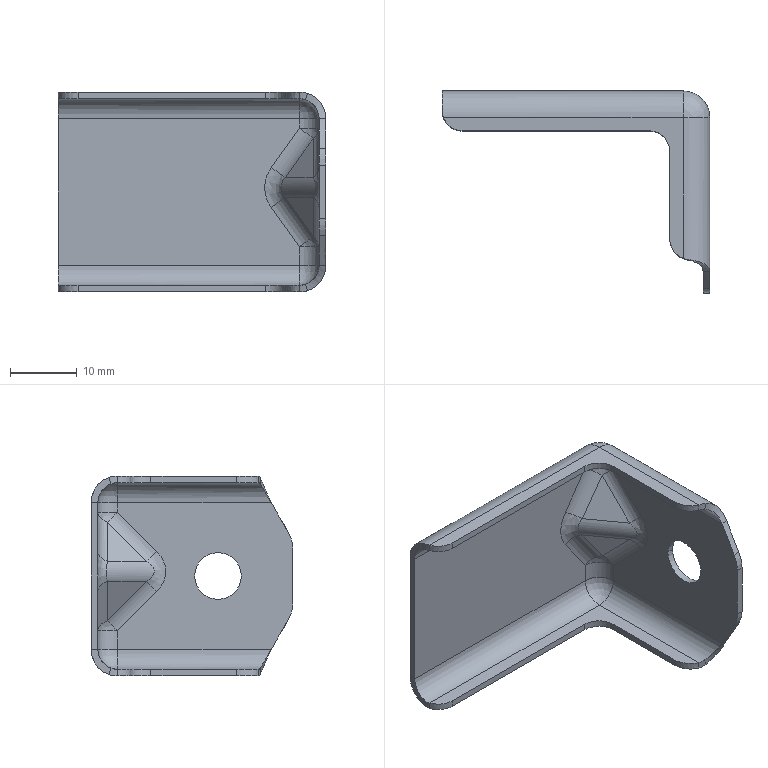Part | STEP file | FNA5401191 | 1 solid | 72 faces | box 40.165 x 30.291 x 30.011 mm | volume 2314 mm3 | cylinder 30 | plane 20 | spline 14 | sphere 8 | commonest cylinder face diameters 6 x15 8 x10 7 x2 10 x2 4 x1